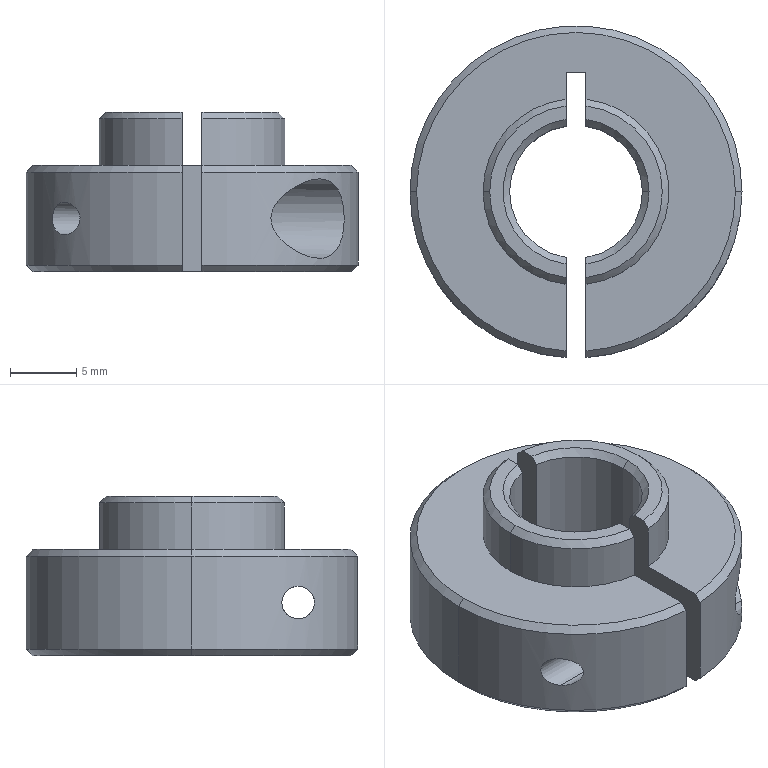Part | STEP file | PN_0001_Z_PSCLSJ10-14_1_Default | 1 solid | 40 faces | box 25 x 24.977 x 12 mm | volume 3181 mm3 | cone 15 | cylinder 15 | plane 10 | commonest cylinder face diameters 10 x3 14 x3 25 x3 2.459 x2 3.5 x2 6 x2